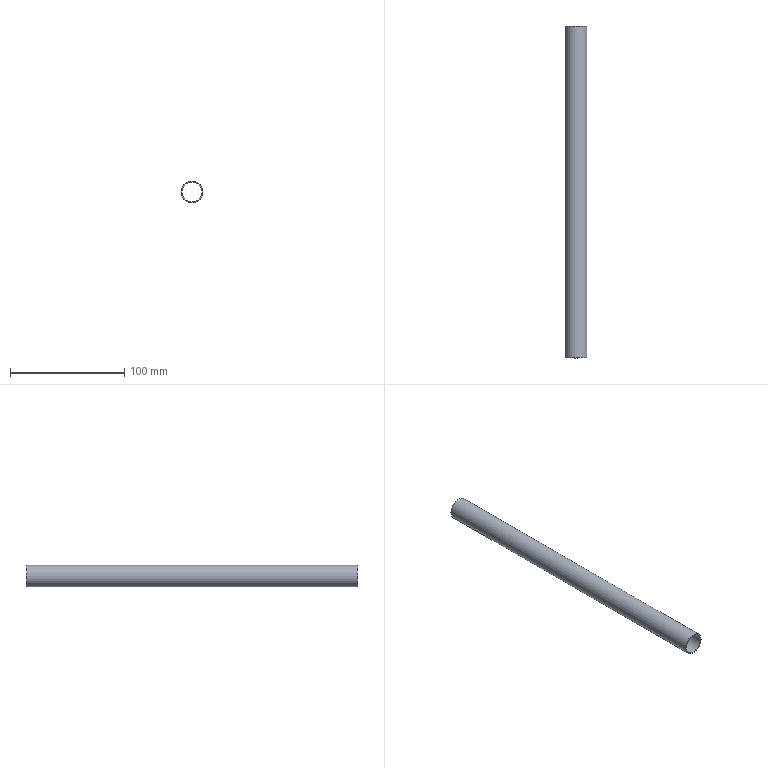Part | STEP file | 1-56.17 | 1 solid | 4 faces | box 19 x 290 x 19 mm | volume 12470 mm3 | plane 2 | cylinder 2 | commonest cylinder face diameters 17.5 x1 19 x1
STEP:
#1=CARTESIAN_POINT('',(0.,0.,0.));
#2=DIRECTION('',(0.,0.,1.));
#3=DIRECTION('',(1.,0.,0.));
#4=AXIS2_PLACEMENT_3D('',#1,#2,#3);
#5=CARTESIAN_POINT('',(9.5,0.,0.));
#6=VERTEX_POINT('',#5);
#7=CARTESIAN_POINT('',(0.,0.,0.));
#8=DIRECTION('',(0.,-1.,0.));
#9=DIRECTION('',(1.,0.,0.));
#10=AXIS2_PLACEMENT_3D('',#7,#8,#9);
#11=CIRCLE('',#10,9.5);
#12=CARTESIAN_POINT('',(-2.546,0.,0.));
#13=DIRECTION('',(0.,-1.,0.));
#14=DIRECTION('',(1.,0.,0.));
#15=AXIS2_PLACEMENT_3D('',#12,#13,#14);
#16=PLANE('',#15);
#17=CARTESIAN_POINT('',(2.546,0.));
#18=DIRECTION('',(1.,0.));
#19=AXIS2_PLACEMENT_2D('',#17,#18);
#20=CIRCLE('',#19,9.5);
#21=(GEOMETRIC_REPRESENTATION_CONTEXT(2)PARAMETRIC_REPRESENTATION_CONTEXT()REPRESENTATION_CONTEXT('',''));
#22=DEFINITIONAL_REPRESENTATION('',(#20),#21);
#23=PCURVE('',#16,#22);
#24=CARTESIAN_POINT('',(0.,0.,0.));
#25=DIRECTION('',(0.,1.,0.));
#26=DIRECTION('',(1.,0.,0.));
#27=AXIS2_PLACEMENT_3D('',#24,#25,#26);
#28=CYLINDRICAL_SURFACE('',#27,9.5);
#29=CARTESIAN_POINT('',(6.283,0.));
#30=DIRECTION('',(-1.,0.));
#31=VECTOR('',#30,1.);
#32=LINE('',#29,#31);
#33=(GEOMETRIC_REPRESENTATION_CONTEXT(2)PARAMETRIC_REPRESENTATION_CONTEXT()REPRESENTATION_CONTEXT('',''));
#34=DEFINITIONAL_REPRESENTATION('',(#32),#33);
#35=PCURVE('',#28,#34);
#36=SURFACE_CURVE('',#11,(#23,#35),.PCURVE_S1.);
#37=EDGE_CURVE('',#6,#6,#36,.T.);
#38=ORIENTED_EDGE('',*,*,#37,.T.);
#39=EDGE_LOOP('',(#38));
#40=FACE_BOUND('',#39,.T.);
#41=CARTESIAN_POINT('',(8.75,0.,0.));
#42=VERTEX_POINT('',#41);
#43=CARTESIAN_POINT('',(0.,0.,0.));
#44=DIRECTION('',(0.,1.,0.));
#45=DIRECTION('',(1.,0.,0.));
#46=AXIS2_PLACEMENT_3D('',#43,#44,#45);
#47=CIRCLE('',#46,8.75);
#48=CARTESIAN_POINT('',(11.296,0.));
#49=CARTESIAN_POINT('',(11.296,-15.155));
#50=CARTESIAN_POINT('',(-1.829,-7.578));
#51=CARTESIAN_POINT('',(-14.954,0.));
#52=CARTESIAN_POINT('',(-1.829,7.578));
#53=CARTESIAN_POINT('',(11.296,15.155));
#54=CARTESIAN_POINT('',(11.296,0.));
#55=(BOUNDED_CURVE()B_SPLINE_CURVE(2,(#48,#49,#50,#51,#52,#53,#54),.UNSPECIFIED.,.T.,.F.)B_SPLINE_CURVE_WITH_KNOTS((1,2,2,2,2,1),(-2.094,0.,2.094,4.189,6.283,8.378),.UNSPECIFIED.)CURVE()GEOMETRIC_REPRESENTATION_ITEM()RATIONAL_B_SPLINE_CURVE((1.,0.5,1.,0.5,1.,0.5,1.))REPRESENTATION_ITEM(''));
#56=(GEOMETRIC_REPRESENTATION_CONTEXT(2)PARAMETRIC_REPRESENTATION_CONTEXT()REPRESENTATION_CONTEXT('',''));
#57=DEFINITIONAL_REPRESENTATION('',(#55),#56);
#58=PCURVE('',#16,#57);
#59=CARTESIAN_POINT('',(0.,0.,0.));
#60=DIRECTION('',(0.,1.,0.));
#61=DIRECTION('',(1.,0.,0.));
#62=AXIS2_PLACEMENT_3D('',#59,#60,#61);
#63=CYLINDRICAL_SURFACE('',#62,8.75);
#64=CARTESIAN_POINT('',(0.,0.));
#65=DIRECTION('',(1.,0.));
#66=VECTOR('',#65,1.);
#67=LINE('',#64,#66);
#68=(GEOMETRIC_REPRESENTATION_CONTEXT(2)PARAMETRIC_REPRESENTATION_CONTEXT()REPRESENTATION_CONTEXT('',''));
#69=DEFINITIONAL_REPRESENTATION('',(#67),#68);
#70=PCURVE('',#63,#69);
#71=SURFACE_CURVE('',#47,(#58,#70),.PCURVE_S1.);
#72=EDGE_CURVE('',#42,#42,#71,.T.);
#73=ORIENTED_EDGE('',*,*,#72,.T.);
#74=EDGE_LOOP('',(#73));
#75=FACE_BOUND('',#74,.T.);
#76=ADVANCED_FACE('',(#40,#75),#16,.T.);
#77=CARTESIAN_POINT('',(9.5,290.,0.));
#78=VERTEX_POINT('',#77);
#79=CARTESIAN_POINT('',(0.,290.,0.));
#80=DIRECTION('',(0.,-1.,0.));
#81=DIRECTION('',(1.,0.,0.));
#82=AXIS2_PLACEMENT_3D('',#79,#80,#81);
#83=CIRCLE('',#82,9.5);
#84=CARTESIAN_POINT('',(-2.546,290.,0.));
#85=DIRECTION('',(0.,-1.,0.));
#86=DIRECTION('',(1.,0.,0.));
#87=AXIS2_PLACEMENT_3D('',#84,#85,#86);
#88=PLANE('',#87);
#89=CARTESIAN_POINT('',(2.546,0.));
#90=DIRECTION('',(1.,0.));
#91=AXIS2_PLACEMENT_2D('',#89,#90);
#92=CIRCLE('',#91,9.5);
#93=(GEOMETRIC_REPRESENTATION_CONTEXT(2)PARAMETRIC_REPRESENTATION_CONTEXT()REPRESENTATION_CONTEXT('',''));
#94=DEFINITIONAL_REPRESENTATION('',(#92),#93);
#95=PCURVE('',#88,#94);
#96=CARTESIAN_POINT('',(6.283,290.));
#97=DIRECTION('',(-1.,0.));
#98=VECTOR('',#97,1.);
#99=LINE('',#96,#98);
#100=(GEOMETRIC_REPRESENTATION_CONTEXT(2)PARAMETRIC_REPRESENTATION_CONTEXT()REPRESENTATION_CONTEXT('',''));
#101=DEFINITIONAL_REPRESENTATION('',(#99),#100);
#102=PCURVE('',#28,#101);
#103=SURFACE_CURVE('',#83,(#95,#102),.PCURVE_S1.);
#104=EDGE_CURVE('',#78,#78,#103,.T.);
#105=ORIENTED_EDGE('',*,*,#104,.T.);
#106=EDGE_LOOP('',(#105));
#107=FACE_BOUND('',#106,.F.);
#108=CARTESIAN_POINT('',(8.75,290.,0.));
#109=VERTEX_POINT('',#108);
#110=CARTESIAN_POINT('',(0.,290.,0.));
#111=DIRECTION('',(0.,1.,0.));
#112=DIRECTION('',(1.,0.,0.));
#113=AXIS2_PLACEMENT_3D('',#110,#111,#112);
#114=CIRCLE('',#113,8.75);
#115=CARTESIAN_POINT('',(11.296,0.));
#116=CARTESIAN_POINT('',(11.296,-15.155));
#117=CARTESIAN_POINT('',(-1.829,-7.578));
#118=CARTESIAN_POINT('',(-14.954,0.));
#119=CARTESIAN_POINT('',(-1.829,7.578));
#120=CARTESIAN_POINT('',(11.296,15.155));
#121=CARTESIAN_POINT('',(11.296,0.));
#122=(BOUNDED_CURVE()B_SPLINE_CURVE(2,(#115,#116,#117,#118,#119,#120,#121),.UNSPECIFIED.,.T.,.F.)B_SPLINE_CURVE_WITH_KNOTS((1,2,2,2,2,1),(-2.094,0.,2.094,4.189,6.283,8.378),.UNSPECIFIED.)CURVE()GEOMETRIC_REPRESENTATION_ITEM()RATIONAL_B_SPLINE_CURVE((1.,0.5,1.,0.5,1.,0.5,1.))REPRESENTATION_ITEM(''));
#123=(GEOMETRIC_REPRESENTATION_CONTEXT(2)PARAMETRIC_REPRESENTATION_CONTEXT()REPRESENTATION_CONTEXT('',''));
#124=DEFINITIONAL_REPRESENTATION('',(#122),#123);
#125=PCURVE('',#88,#124);
#126=CARTESIAN_POINT('',(0.,290.));
#127=DIRECTION('',(1.,0.));
#128=VECTOR('',#127,1.);
#129=LINE('',#126,#128);
#130=(GEOMETRIC_REPRESENTATION_CONTEXT(2)PARAMETRIC_REPRESENTATION_CONTEXT()REPRESENTATION_CONTEXT('',''));
#131=DEFINITIONAL_REPRESENTATION('',(#129),#130);
#132=PCURVE('',#63,#131);
#133=SURFACE_CURVE('',#114,(#125,#132),.PCURVE_S1.);
#134=EDGE_CURVE('',#109,#109,#133,.T.);
#135=ORIENTED_EDGE('',*,*,#134,.T.);
#136=EDGE_LOOP('',(#135));
#137=FACE_BOUND('',#136,.F.);
#138=ADVANCED_FACE('',(#107,#137),#88,.F.);
#139=CARTESIAN_POINT('',(9.5,0.,0.));
#140=DIRECTION('',(0.,1.,0.));
#141=VECTOR('',#140,1.);
#142=LINE('',#139,#141);
#143=CARTESIAN_POINT('',(6.283,0.));
#144=DIRECTION('',(0.,1.));
#145=VECTOR('',#144,1.);
#146=LINE('',#143,#145);
#147=(GEOMETRIC_REPRESENTATION_CONTEXT(2)PARAMETRIC_REPRESENTATION_CONTEXT()REPRESENTATION_CONTEXT('',''));
#148=DEFINITIONAL_REPRESENTATION('',(#146),#147);
#149=PCURVE('',#28,#148);
#150=CARTESIAN_POINT('',(0.,0.));
#151=DIRECTION('',(0.,1.));
#152=VECTOR('',#151,1.);
#153=LINE('',#150,#152);
#154=(GEOMETRIC_REPRESENTATION_CONTEXT(2)PARAMETRIC_REPRESENTATION_CONTEXT()REPRESENTATION_CONTEXT('',''));
#155=DEFINITIONAL_REPRESENTATION('',(#153),#154);
#156=PCURVE('',#28,#155);
#157=SEAM_CURVE('',#142,(#149,#156),.PCURVE_S1.);
#158=EDGE_CURVE('',#6,#78,#157,.T.);
#159=ORIENTED_EDGE('',*,*,#158,.T.);
#160=ORIENTED_EDGE('',*,*,#104,.T.);
#161=ORIENTED_EDGE('',*,*,#158,.F.);
#162=ORIENTED_EDGE('',*,*,#37,.F.);
#163=EDGE_LOOP('',(#159,#160,#161,#162));
#164=FACE_BOUND('',#163,.T.);
#165=ADVANCED_FACE('',(#164),#28,.T.);
#166=ORIENTED_EDGE('',*,*,#72,.T.);
#167=CARTESIAN_POINT('',(8.75,0.,0.));
#168=DIRECTION('',(0.,1.,0.));
#169=VECTOR('',#168,1.);
#170=LINE('',#167,#169);
#171=CARTESIAN_POINT('',(6.283,0.));
#172=DIRECTION('',(0.,1.));
#173=VECTOR('',#172,1.);
#174=LINE('',#171,#173);
#175=(GEOMETRIC_REPRESENTATION_CONTEXT(2)PARAMETRIC_REPRESENTATION_CONTEXT()REPRESENTATION_CONTEXT('',''));
#176=DEFINITIONAL_REPRESENTATION('',(#174),#175);
#177=PCURVE('',#63,#176);
#178=CARTESIAN_POINT('',(0.,0.));
#179=DIRECTION('',(0.,1.));
#180=VECTOR('',#179,1.);
#181=LINE('',#178,#180);
#182=(GEOMETRIC_REPRESENTATION_CONTEXT(2)PARAMETRIC_REPRESENTATION_CONTEXT()REPRESENTATION_CONTEXT('',''));
#183=DEFINITIONAL_REPRESENTATION('',(#181),#182);
#184=PCURVE('',#63,#183);
#185=SEAM_CURVE('',#170,(#177,#184),.PCURVE_S1.);
#186=EDGE_CURVE('',#42,#109,#185,.T.);
#187=ORIENTED_EDGE('',*,*,#186,.T.);
#188=ORIENTED_EDGE('',*,*,#134,.F.);
#189=ORIENTED_EDGE('',*,*,#186,.F.);
#190=EDGE_LOOP('',(#166,#187,#188,#189));
#191=FACE_BOUND('',#190,.F.);
#192=ADVANCED_FACE('',(#191),#63,.F.);
#193=CLOSED_SHELL('',(#76,#138,#165,#192));
#194=MANIFOLD_SOLID_BREP('',#193);
#195=(LENGTH_UNIT()NAMED_UNIT(*)SI_UNIT(.MILLI.,.METRE.));
#196=UNCERTAINTY_MEASURE_WITH_UNIT(LENGTH_MEASURE(0.0000001),#195,'','');
#197=(NAMED_UNIT(*)PLANE_ANGLE_UNIT()SI_UNIT($,.RADIAN.));
#198=(NAMED_UNIT(*)SI_UNIT($,.STERADIAN.)SOLID_ANGLE_UNIT());
#199=(GEOMETRIC_REPRESENTATION_CONTEXT(3)GLOBAL_UNCERTAINTY_ASSIGNED_CONTEXT((#196))GLOBAL_UNIT_ASSIGNED_CONTEXT((#195,#197,#198))REPRESENTATION_CONTEXT('',''));
#200=ADVANCED_BREP_SHAPE_REPRESENTATION('',(#4,#194),#199);